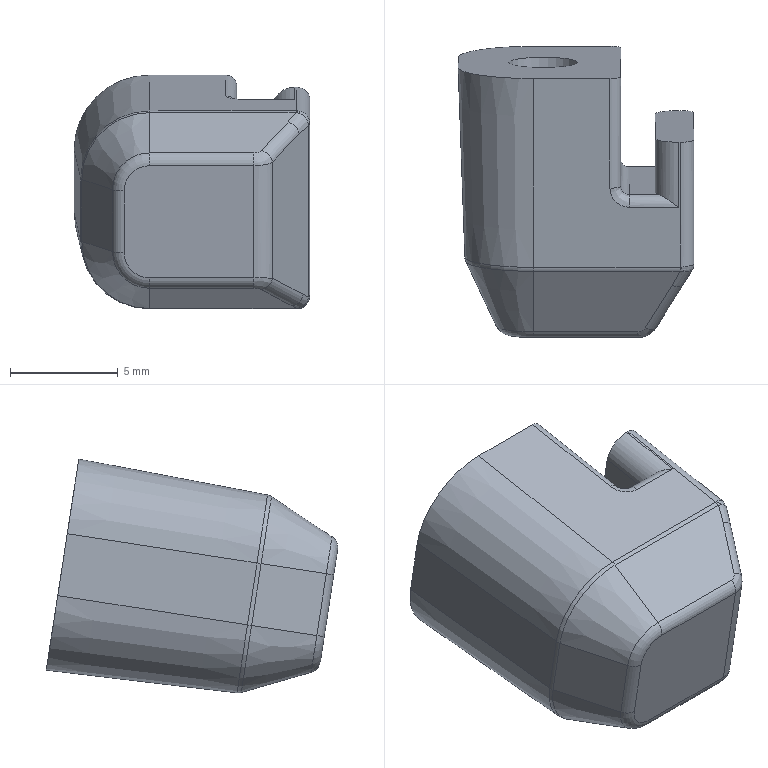Part | SolidWorks | features BaseBody 1 | 1 solid | 56 faces | box 10.93 x 13.517 x 10.84 mm | volume 889.407 mm3 | cylinder 21 | plane 15 | spline 12 | torus 4 | cone 4 | commonest cylinder face diameters 1 x8 1.2 x7 2.2 x2 3.2 x2 0.8 x1 2 x1